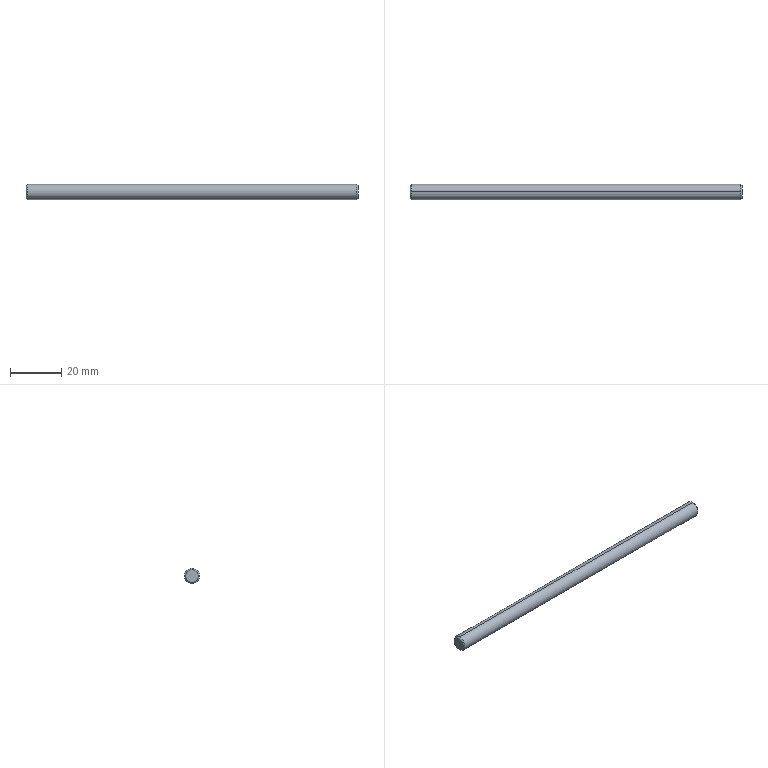Part | SolidWorks | features Chamfer 1, Revolution 1 | 1 solid | 8 faces | box 130 x 6 x 6 mm | volume 3671 mm3 | cone 4 | cylinder 2 | plane 2 | commonest cylinder face diameters 6 x2
STEP:
#1=CARTESIAN_POINT('',(0.,0.,2.5));
#2=VERTEX_POINT('',#1);
#3=CARTESIAN_POINT('',(0.,0.,-2.5));
#4=VERTEX_POINT('',#3);
#5=CARTESIAN_POINT('',(0.,0.,0.));
#6=DIRECTION('',(-1.,0.,0.));
#7=DIRECTION('',(0.,0.,-1.));
#8=AXIS2_PLACEMENT_3D('',#5,#6,#7);
#9=CIRCLE('',#8,2.5);
#10=EDGE_CURVE('',#2,#4,#9,.T.);
#11=ORIENTED_EDGE('',*,*,#10,.F.);
#12=CARTESIAN_POINT('',(0.5,0.,3.));
#13=VERTEX_POINT('',#12);
#14=CARTESIAN_POINT('',(0.,0.,2.5));
#15=DIRECTION('',(0.7071,0.,0.7071));
#16=VECTOR('',#15,1000.);
#17=LINE('',#14,#16);
#18=EDGE_CURVE('',#2,#13,#17,.T.);
#19=ORIENTED_EDGE('',*,*,#18,.T.);
#20=CARTESIAN_POINT('',(0.5,0.,-3.));
#21=VERTEX_POINT('',#20);
#22=CARTESIAN_POINT('',(0.5,0.,0.));
#23=DIRECTION('',(1.,0.,0.));
#24=DIRECTION('',(0.,0.,-1.));
#25=AXIS2_PLACEMENT_3D('',#22,#23,#24);
#26=CIRCLE('',#25,3.);
#27=EDGE_CURVE('',#21,#13,#26,.T.);
#28=ORIENTED_EDGE('',*,*,#27,.F.);
#29=CARTESIAN_POINT('',(0.,0.,-2.5));
#30=DIRECTION('',(0.7071,0.,-0.7071));
#31=VECTOR('',#30,1000.);
#32=LINE('',#29,#31);
#33=EDGE_CURVE('',#4,#21,#32,.T.);
#34=ORIENTED_EDGE('',*,*,#33,.F.);
#35=EDGE_LOOP('',(#11,#19,#28,#34));
#36=FACE_OUTER_BOUND('',#35,.T.);
#37=CARTESIAN_POINT('',(0.,0.,0.));
#38=DIRECTION('',(1.,0.,0.));
#39=DIRECTION('',(0.,0.,-1.));
#40=AXIS2_PLACEMENT_3D('',#37,#38,#39);
#41=CONICAL_SURFACE('',#40,2.5,0.7854);
#42=ADVANCED_FACE('',(#36),#41,.T.);
#43=CARTESIAN_POINT('',(130.,0.,-2.5));
#44=VERTEX_POINT('',#43);
#45=CARTESIAN_POINT('',(130.,0.,2.5));
#46=VERTEX_POINT('',#45);
#47=CARTESIAN_POINT('',(130.,0.,0.));
#48=DIRECTION('',(1.,0.,0.));
#49=DIRECTION('',(0.,0.,1.));
#50=AXIS2_PLACEMENT_3D('',#47,#48,#49);
#51=CIRCLE('',#50,2.5);
#52=EDGE_CURVE('',#44,#46,#51,.T.);
#53=ORIENTED_EDGE('',*,*,#52,.F.);
#54=CARTESIAN_POINT('',(129.5,0.,-3.));
#55=VERTEX_POINT('',#54);
#56=CARTESIAN_POINT('',(129.5,0.,-3.));
#57=DIRECTION('',(-0.7071,0.,-0.7071));
#58=VECTOR('',#57,1000.);
#59=LINE('',#56,#58);
#60=EDGE_CURVE('',#44,#55,#59,.T.);
#61=ORIENTED_EDGE('',*,*,#60,.T.);
#62=CARTESIAN_POINT('',(129.5,0.,3.));
#63=VERTEX_POINT('',#62);
#64=CARTESIAN_POINT('',(129.5,0.,0.));
#65=DIRECTION('',(-1.,0.,0.));
#66=DIRECTION('',(0.,0.,1.));
#67=AXIS2_PLACEMENT_3D('',#64,#65,#66);
#68=CIRCLE('',#67,3.);
#69=EDGE_CURVE('',#63,#55,#68,.T.);
#70=ORIENTED_EDGE('',*,*,#69,.F.);
#71=CARTESIAN_POINT('',(129.5,0.,3.));
#72=DIRECTION('',(-0.7071,0.,0.7071));
#73=VECTOR('',#72,1000.);
#74=LINE('',#71,#73);
#75=EDGE_CURVE('',#46,#63,#74,.T.);
#76=ORIENTED_EDGE('',*,*,#75,.F.);
#77=EDGE_LOOP('',(#53,#61,#70,#76));
#78=FACE_OUTER_BOUND('',#77,.T.);
#79=CARTESIAN_POINT('',(129.5,0.,0.));
#80=DIRECTION('',(-1.,0.,0.));
#81=DIRECTION('',(0.,0.,1.));
#82=AXIS2_PLACEMENT_3D('',#79,#80,#81);
#83=CONICAL_SURFACE('',#82,3.,0.7854);
#84=ADVANCED_FACE('',(#78),#83,.T.);
#85=ORIENTED_EDGE('',*,*,#69,.T.);
#86=CARTESIAN_POINT('',(0.,0.,-3.));
#87=DIRECTION('',(-1.,0.,0.));
#88=VECTOR('',#87,1000.);
#89=LINE('',#86,#88);
#90=EDGE_CURVE('',#55,#21,#89,.T.);
#91=ORIENTED_EDGE('',*,*,#90,.T.);
#92=ORIENTED_EDGE('',*,*,#27,.T.);
#93=CARTESIAN_POINT('',(0.,0.,3.));
#94=DIRECTION('',(-1.,0.,0.));
#95=VECTOR('',#94,1000.);
#96=LINE('',#93,#95);
#97=EDGE_CURVE('',#63,#13,#96,.T.);
#98=ORIENTED_EDGE('',*,*,#97,.F.);
#99=EDGE_LOOP('',(#85,#91,#92,#98));
#100=FACE_OUTER_BOUND('',#99,.T.);
#101=CARTESIAN_POINT('',(0.,0.,0.));
#102=DIRECTION('',(-1.,0.,0.));
#103=DIRECTION('',(0.,0.,1.));
#104=AXIS2_PLACEMENT_3D('',#101,#102,#103);
#105=CYLINDRICAL_SURFACE('',#104,3.);
#106=ADVANCED_FACE('',(#100),#105,.T.);
#107=CARTESIAN_POINT('',(0.,0.,0.));
#108=DIRECTION('',(-1.,0.,0.));
#109=DIRECTION('',(0.,0.,-1.));
#110=AXIS2_PLACEMENT_3D('',#107,#108,#109);
#111=CIRCLE('',#110,2.5);
#112=EDGE_CURVE('',#4,#2,#111,.T.);
#113=ORIENTED_EDGE('',*,*,#112,.T.);
#114=ORIENTED_EDGE('',*,*,#10,.T.);
#115=EDGE_LOOP('',(#113,#114));
#116=FACE_OUTER_BOUND('',#115,.T.);
#117=CARTESIAN_POINT('',(0.,0.,0.));
#118=DIRECTION('',(1.,0.,0.));
#119=DIRECTION('',(0.,0.,-1.));
#120=AXIS2_PLACEMENT_3D('',#117,#118,#119);
#121=PLANE('',#120);
#122=ADVANCED_FACE('',(#116),#121,.F.);
#123=ORIENTED_EDGE('',*,*,#90,.F.);
#124=CARTESIAN_POINT('',(129.5,0.,0.));
#125=DIRECTION('',(-1.,0.,0.));
#126=DIRECTION('',(0.,0.,1.));
#127=AXIS2_PLACEMENT_3D('',#124,#125,#126);
#128=CIRCLE('',#127,3.);
#129=EDGE_CURVE('',#55,#63,#128,.T.);
#130=ORIENTED_EDGE('',*,*,#129,.T.);
#131=ORIENTED_EDGE('',*,*,#97,.T.);
#132=CARTESIAN_POINT('',(0.5,0.,0.));
#133=DIRECTION('',(1.,0.,0.));
#134=DIRECTION('',(0.,0.,-1.));
#135=AXIS2_PLACEMENT_3D('',#132,#133,#134);
#136=CIRCLE('',#135,3.);
#137=EDGE_CURVE('',#13,#21,#136,.T.);
#138=ORIENTED_EDGE('',*,*,#137,.T.);
#139=EDGE_LOOP('',(#123,#130,#131,#138));
#140=FACE_OUTER_BOUND('',#139,.T.);
#141=CARTESIAN_POINT('',(0.,0.,0.));
#142=DIRECTION('',(-1.,0.,0.));
#143=DIRECTION('',(0.,0.,1.));
#144=AXIS2_PLACEMENT_3D('',#141,#142,#143);
#145=CYLINDRICAL_SURFACE('',#144,3.);
#146=ADVANCED_FACE('',(#140),#145,.T.);
#147=CARTESIAN_POINT('',(130.,0.,0.));
#148=DIRECTION('',(1.,0.,0.));
#149=DIRECTION('',(0.,0.,1.));
#150=AXIS2_PLACEMENT_3D('',#147,#148,#149);
#151=CIRCLE('',#150,2.5);
#152=EDGE_CURVE('',#46,#44,#151,.T.);
#153=ORIENTED_EDGE('',*,*,#152,.T.);
#154=ORIENTED_EDGE('',*,*,#52,.T.);
#155=EDGE_LOOP('',(#153,#154));
#156=FACE_OUTER_BOUND('',#155,.T.);
#157=CARTESIAN_POINT('',(130.,0.,0.));
#158=DIRECTION('',(-1.,0.,0.));
#159=DIRECTION('',(0.,0.,1.));
#160=AXIS2_PLACEMENT_3D('',#157,#158,#159);
#161=PLANE('',#160);
#162=ADVANCED_FACE('',(#156),#161,.F.);
#163=ORIENTED_EDGE('',*,*,#60,.F.);
#164=ORIENTED_EDGE('',*,*,#152,.F.);
#165=ORIENTED_EDGE('',*,*,#75,.T.);
#166=ORIENTED_EDGE('',*,*,#129,.F.);
#167=EDGE_LOOP('',(#163,#164,#165,#166));
#168=FACE_OUTER_BOUND('',#167,.T.);
#169=CARTESIAN_POINT('',(129.5,0.,0.));
#170=DIRECTION('',(-1.,0.,0.));
#171=DIRECTION('',(0.,0.,1.));
#172=AXIS2_PLACEMENT_3D('',#169,#170,#171);
#173=CONICAL_SURFACE('',#172,3.,0.7854);
#174=ADVANCED_FACE('',(#168),#173,.T.);
#175=ORIENTED_EDGE('',*,*,#18,.F.);
#176=ORIENTED_EDGE('',*,*,#112,.F.);
#177=ORIENTED_EDGE('',*,*,#33,.T.);
#178=ORIENTED_EDGE('',*,*,#137,.F.);
#179=EDGE_LOOP('',(#175,#176,#177,#178));
#180=FACE_OUTER_BOUND('',#179,.T.);
#181=CARTESIAN_POINT('',(0.,0.,0.));
#182=DIRECTION('',(1.,0.,0.));
#183=DIRECTION('',(0.,0.,-1.));
#184=AXIS2_PLACEMENT_3D('',#181,#182,#183);
#185=CONICAL_SURFACE('',#184,2.5,0.7854);
#186=ADVANCED_FACE('',(#180),#185,.T.);
#187=CLOSED_SHELL('',(#42,#84,#106,#122,#146,#162,#174,#186));
#188=MANIFOLD_SOLID_BREP('',#187);
#189=CARTESIAN_POINT('',(0.,0.,0.));
#190=DIRECTION('',(0.,0.,1.));
#191=DIRECTION('',(1.,0.,0.));
#192=AXIS2_PLACEMENT_3D('',#189,#190,#191);
#193=(LENGTH_UNIT()NAMED_UNIT(*)SI_UNIT(.MILLI.,.METRE.));
#194=UNCERTAINTY_MEASURE_WITH_UNIT(LENGTH_MEASURE(0.00001),#193,'','');
#195=(NAMED_UNIT(*)PLANE_ANGLE_UNIT()SI_UNIT($,.RADIAN.));
#196=(NAMED_UNIT(*)SI_UNIT($,.STERADIAN.)SOLID_ANGLE_UNIT());
#197=(GEOMETRIC_REPRESENTATION_CONTEXT(3)GLOBAL_UNCERTAINTY_ASSIGNED_CONTEXT((#194))GLOBAL_UNIT_ASSIGNED_CONTEXT((#193,#195,#196))REPRESENTATION_CONTEXT('',''));
#198=ADVANCED_BREP_SHAPE_REPRESENTATION('',(#188,#192),#197);